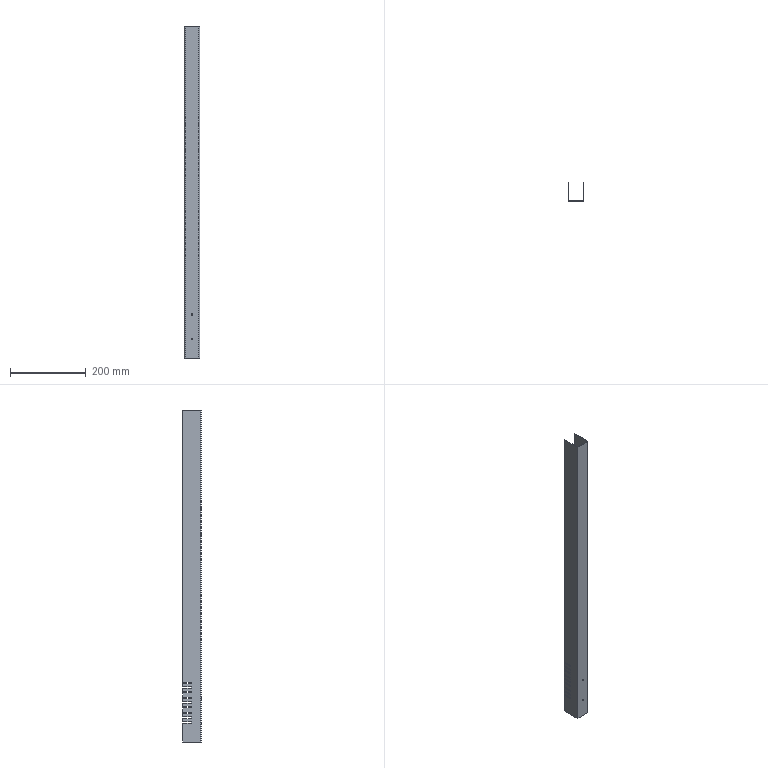Part | SolidWorks | features MoveFace 2, Cut 1, FlatPattern 1, ICE 1, LPattern 1, SMBaseFlange 1, SheetMetal 1 | 1 solid | 98 faces | box 40 x 50 x 876 mm | volume 176360 mm3 | plane 90 | cylinder 8 | commonest cylinder face diameters 5 x4 0.4 x2 3.4 x2